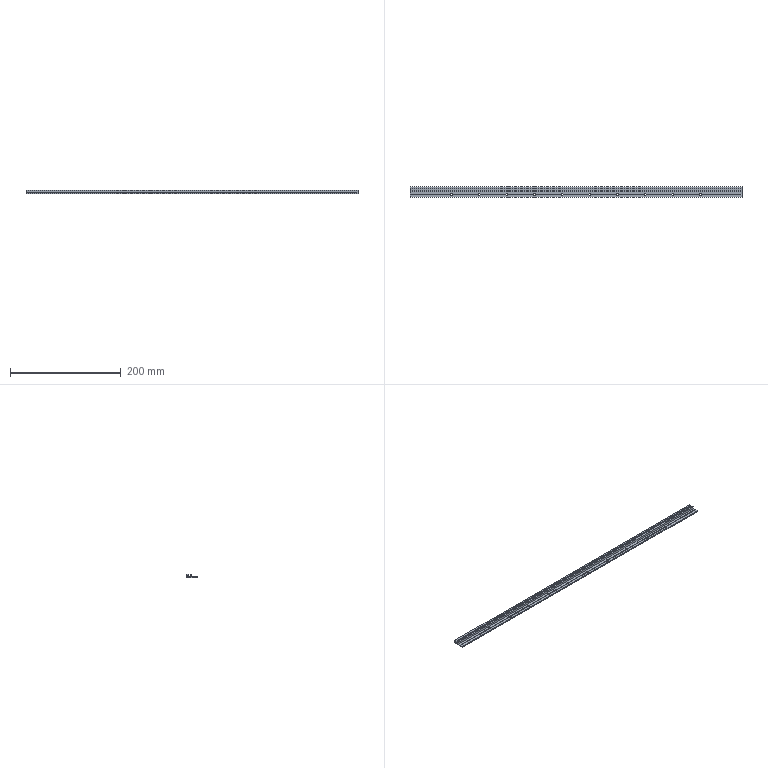Part | STEP file | SENC3-600-LX45-590_lx | 1 solid | 49 faces | box 600 x 19 x 6 mm | volume 30746 mm3 | plane 39 | cylinder 10 | commonest cylinder face diameters 3.5 x10